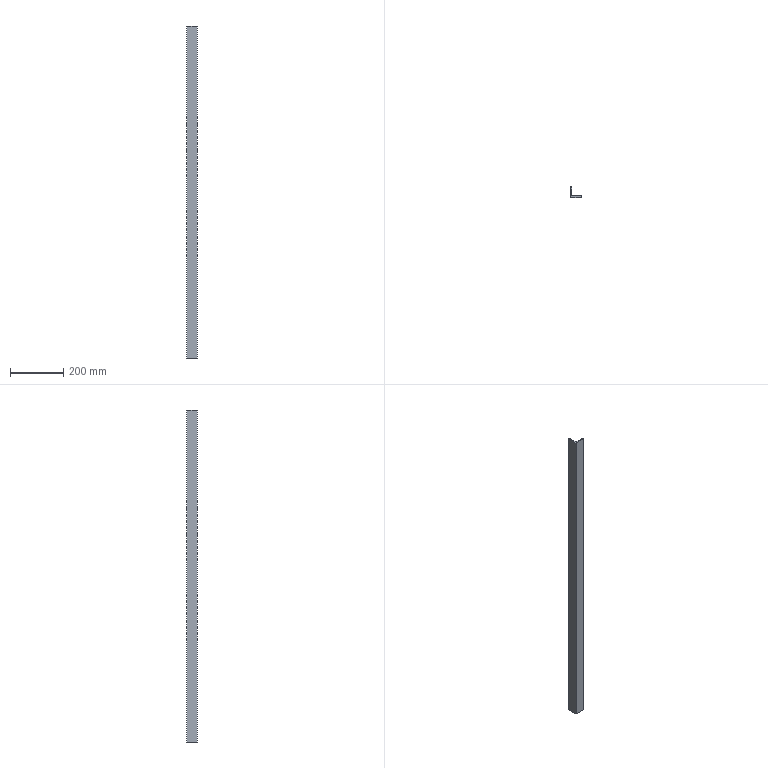Part | SolidWorks | features ICE 1, LibraryFeature 1 | 1 solid | 11 faces | box 40 x 40 x 1250 mm | volume 385753 mm3 | plane 8 | cylinder 3 | commonest cylinder face diameters 2.667 x2 10 x1
STEP:
#1=CARTESIAN_POINT('',(9.,4.,-625.));
#2=VERTEX_POINT('',#1);
#3=CARTESIAN_POINT('',(4.,9.,-625.));
#4=VERTEX_POINT('',#3);
#5=CARTESIAN_POINT('',(9.,9.,-625.));
#6=DIRECTION('',(0.,0.,-1.));
#7=DIRECTION('',(-1.,0.,0.));
#8=AXIS2_PLACEMENT_3D('',#5,#6,#7);
#9=CIRCLE('',#8,5.);
#10=EDGE_CURVE('',#2,#4,#9,.T.);
#11=ORIENTED_EDGE('',*,*,#10,.T.);
#12=CARTESIAN_POINT('',(4.,9.,625.));
#13=VERTEX_POINT('',#12);
#14=CARTESIAN_POINT('',(4.,9.,625.));
#15=DIRECTION('',(0.,0.,-1.));
#16=VECTOR('',#15,1000.);
#17=LINE('',#14,#16);
#18=EDGE_CURVE('',#13,#4,#17,.T.);
#19=ORIENTED_EDGE('',*,*,#18,.F.);
#20=CARTESIAN_POINT('',(9.,4.,625.));
#21=VERTEX_POINT('',#20);
#22=CARTESIAN_POINT('',(9.,9.,625.));
#23=DIRECTION('',(0.,0.,-1.));
#24=DIRECTION('',(-1.,0.,0.));
#25=AXIS2_PLACEMENT_3D('',#22,#23,#24);
#26=CIRCLE('',#25,5.);
#27=EDGE_CURVE('',#21,#13,#26,.T.);
#28=ORIENTED_EDGE('',*,*,#27,.F.);
#29=CARTESIAN_POINT('',(9.,4.,625.));
#30=DIRECTION('',(0.,0.,-1.));
#31=VECTOR('',#30,1000.);
#32=LINE('',#29,#31);
#33=EDGE_CURVE('',#21,#2,#32,.T.);
#34=ORIENTED_EDGE('',*,*,#33,.T.);
#35=EDGE_LOOP('',(#11,#19,#28,#34));
#36=FACE_OUTER_BOUND('',#35,.T.);
#37=CARTESIAN_POINT('',(9.,9.,625.));
#38=DIRECTION('',(0.,0.,-1.));
#39=DIRECTION('',(-1.,0.,0.));
#40=AXIS2_PLACEMENT_3D('',#37,#38,#39);
#41=CYLINDRICAL_SURFACE('',#40,5.);
#42=ADVANCED_FACE('',(#36),#41,.F.);
#43=CARTESIAN_POINT('',(4.,38.667,-625.));
#44=VERTEX_POINT('',#43);
#45=CARTESIAN_POINT('',(4.,38.667,-625.));
#46=DIRECTION('',(0.,-1.,0.));
#47=VECTOR('',#46,1000.);
#48=LINE('',#45,#47);
#49=EDGE_CURVE('',#44,#4,#48,.T.);
#50=ORIENTED_EDGE('',*,*,#49,.F.);
#51=CARTESIAN_POINT('',(4.,38.667,625.));
#52=VERTEX_POINT('',#51);
#53=CARTESIAN_POINT('',(4.,38.667,625.));
#54=DIRECTION('',(0.,0.,-1.));
#55=VECTOR('',#54,1000.);
#56=LINE('',#53,#55);
#57=EDGE_CURVE('',#52,#44,#56,.T.);
#58=ORIENTED_EDGE('',*,*,#57,.F.);
#59=CARTESIAN_POINT('',(4.,38.667,625.));
#60=DIRECTION('',(0.,-1.,0.));
#61=VECTOR('',#60,1000.);
#62=LINE('',#59,#61);
#63=EDGE_CURVE('',#52,#13,#62,.T.);
#64=ORIENTED_EDGE('',*,*,#63,.T.);
#65=ORIENTED_EDGE('',*,*,#18,.T.);
#66=EDGE_LOOP('',(#50,#58,#64,#65));
#67=FACE_OUTER_BOUND('',#66,.T.);
#68=CARTESIAN_POINT('',(4.,38.667,625.));
#69=DIRECTION('',(1.,0.,0.));
#70=DIRECTION('',(0.,1.,0.));
#71=AXIS2_PLACEMENT_3D('',#68,#69,#70);
#72=PLANE('',#71);
#73=ADVANCED_FACE('',(#67),#72,.T.);
#74=CARTESIAN_POINT('',(2.667,40.,-625.));
#75=VERTEX_POINT('',#74);
#76=CARTESIAN_POINT('',(2.667,38.667,-625.));
#77=DIRECTION('',(0.,0.,-1.));
#78=DIRECTION('',(-1.,0.,0.));
#79=AXIS2_PLACEMENT_3D('',#76,#77,#78);
#80=CIRCLE('',#79,1.333);
#81=EDGE_CURVE('',#75,#44,#80,.T.);
#82=ORIENTED_EDGE('',*,*,#81,.F.);
#83=CARTESIAN_POINT('',(2.667,40.,625.));
#84=VERTEX_POINT('',#83);
#85=CARTESIAN_POINT('',(2.667,40.,625.));
#86=DIRECTION('',(0.,0.,-1.));
#87=VECTOR('',#86,1000.);
#88=LINE('',#85,#87);
#89=EDGE_CURVE('',#84,#75,#88,.T.);
#90=ORIENTED_EDGE('',*,*,#89,.F.);
#91=CARTESIAN_POINT('',(2.667,38.667,625.));
#92=DIRECTION('',(0.,0.,-1.));
#93=DIRECTION('',(-1.,0.,0.));
#94=AXIS2_PLACEMENT_3D('',#91,#92,#93);
#95=CIRCLE('',#94,1.333);
#96=EDGE_CURVE('',#84,#52,#95,.T.);
#97=ORIENTED_EDGE('',*,*,#96,.T.);
#98=ORIENTED_EDGE('',*,*,#57,.T.);
#99=EDGE_LOOP('',(#82,#90,#97,#98));
#100=FACE_OUTER_BOUND('',#99,.T.);
#101=CARTESIAN_POINT('',(2.667,38.667,625.));
#102=DIRECTION('',(0.,0.,-1.));
#103=DIRECTION('',(-1.,0.,0.));
#104=AXIS2_PLACEMENT_3D('',#101,#102,#103);
#105=CYLINDRICAL_SURFACE('',#104,1.333);
#106=ADVANCED_FACE('',(#100),#105,.T.);
#107=CARTESIAN_POINT('',(0.,40.,-625.));
#108=VERTEX_POINT('',#107);
#109=CARTESIAN_POINT('',(0.,40.,-625.));
#110=DIRECTION('',(1.,0.,0.));
#111=VECTOR('',#110,1000.);
#112=LINE('',#109,#111);
#113=EDGE_CURVE('',#108,#75,#112,.T.);
#114=ORIENTED_EDGE('',*,*,#113,.F.);
#115=CARTESIAN_POINT('',(0.,40.,625.));
#116=VERTEX_POINT('',#115);
#117=CARTESIAN_POINT('',(0.,40.,625.));
#118=DIRECTION('',(0.,0.,-1.));
#119=VECTOR('',#118,1000.);
#120=LINE('',#117,#119);
#121=EDGE_CURVE('',#116,#108,#120,.T.);
#122=ORIENTED_EDGE('',*,*,#121,.F.);
#123=CARTESIAN_POINT('',(0.,40.,625.));
#124=DIRECTION('',(1.,0.,0.));
#125=VECTOR('',#124,1000.);
#126=LINE('',#123,#125);
#127=EDGE_CURVE('',#116,#84,#126,.T.);
#128=ORIENTED_EDGE('',*,*,#127,.T.);
#129=ORIENTED_EDGE('',*,*,#89,.T.);
#130=EDGE_LOOP('',(#114,#122,#128,#129));
#131=FACE_OUTER_BOUND('',#130,.T.);
#132=CARTESIAN_POINT('',(0.,40.,625.));
#133=DIRECTION('',(0.,1.,0.));
#134=DIRECTION('',(0.,0.,1.));
#135=AXIS2_PLACEMENT_3D('',#132,#133,#134);
#136=PLANE('',#135);
#137=ADVANCED_FACE('',(#131),#136,.T.);
#138=CARTESIAN_POINT('',(0.,0.,-625.));
#139=VERTEX_POINT('',#138);
#140=CARTESIAN_POINT('',(0.,0.,-625.));
#141=DIRECTION('',(0.,1.,0.));
#142=VECTOR('',#141,1000.);
#143=LINE('',#140,#142);
#144=EDGE_CURVE('',#139,#108,#143,.T.);
#145=ORIENTED_EDGE('',*,*,#144,.F.);
#146=CARTESIAN_POINT('',(0.,0.,625.));
#147=VERTEX_POINT('',#146);
#148=CARTESIAN_POINT('',(0.,0.,625.));
#149=DIRECTION('',(0.,0.,-1.));
#150=VECTOR('',#149,1000.);
#151=LINE('',#148,#150);
#152=EDGE_CURVE('',#147,#139,#151,.T.);
#153=ORIENTED_EDGE('',*,*,#152,.F.);
#154=CARTESIAN_POINT('',(0.,0.,625.));
#155=DIRECTION('',(0.,1.,0.));
#156=VECTOR('',#155,1000.);
#157=LINE('',#154,#156);
#158=EDGE_CURVE('',#147,#116,#157,.T.);
#159=ORIENTED_EDGE('',*,*,#158,.T.);
#160=ORIENTED_EDGE('',*,*,#121,.T.);
#161=EDGE_LOOP('',(#145,#153,#159,#160));
#162=FACE_OUTER_BOUND('',#161,.T.);
#163=CARTESIAN_POINT('',(0.,0.,625.));
#164=DIRECTION('',(-1.,0.,0.));
#165=DIRECTION('',(0.,0.,1.));
#166=AXIS2_PLACEMENT_3D('',#163,#164,#165);
#167=PLANE('',#166);
#168=ADVANCED_FACE('',(#162),#167,.T.);
#169=CARTESIAN_POINT('',(40.,0.,-625.));
#170=VERTEX_POINT('',#169);
#171=CARTESIAN_POINT('',(40.,0.,-625.));
#172=DIRECTION('',(-1.,0.,0.));
#173=VECTOR('',#172,1000.);
#174=LINE('',#171,#173);
#175=EDGE_CURVE('',#170,#139,#174,.T.);
#176=ORIENTED_EDGE('',*,*,#175,.F.);
#177=CARTESIAN_POINT('',(40.,0.,625.));
#178=VERTEX_POINT('',#177);
#179=CARTESIAN_POINT('',(40.,0.,625.));
#180=DIRECTION('',(0.,0.,-1.));
#181=VECTOR('',#180,1000.);
#182=LINE('',#179,#181);
#183=EDGE_CURVE('',#178,#170,#182,.T.);
#184=ORIENTED_EDGE('',*,*,#183,.F.);
#185=CARTESIAN_POINT('',(40.,0.,625.));
#186=DIRECTION('',(-1.,0.,0.));
#187=VECTOR('',#186,1000.);
#188=LINE('',#185,#187);
#189=EDGE_CURVE('',#178,#147,#188,.T.);
#190=ORIENTED_EDGE('',*,*,#189,.T.);
#191=ORIENTED_EDGE('',*,*,#152,.T.);
#192=EDGE_LOOP('',(#176,#184,#190,#191));
#193=FACE_OUTER_BOUND('',#192,.T.);
#194=CARTESIAN_POINT('',(40.,0.,625.));
#195=DIRECTION('',(0.,-1.,0.));
#196=DIRECTION('',(0.,0.,-1.));
#197=AXIS2_PLACEMENT_3D('',#194,#195,#196);
#198=PLANE('',#197);
#199=ADVANCED_FACE('',(#193),#198,.T.);
#200=CARTESIAN_POINT('',(40.,2.667,-625.));
#201=VERTEX_POINT('',#200);
#202=CARTESIAN_POINT('',(40.,0.,-625.));
#203=DIRECTION('',(0.,1.,0.));
#204=VECTOR('',#203,1000.);
#205=LINE('',#202,#204);
#206=EDGE_CURVE('',#170,#201,#205,.T.);
#207=ORIENTED_EDGE('',*,*,#206,.T.);
#208=CARTESIAN_POINT('',(40.,2.667,625.));
#209=VERTEX_POINT('',#208);
#210=CARTESIAN_POINT('',(40.,2.667,625.));
#211=DIRECTION('',(0.,0.,-1.));
#212=VECTOR('',#211,1000.);
#213=LINE('',#210,#212);
#214=EDGE_CURVE('',#209,#201,#213,.T.);
#215=ORIENTED_EDGE('',*,*,#214,.F.);
#216=CARTESIAN_POINT('',(40.,0.,625.));
#217=DIRECTION('',(0.,1.,0.));
#218=VECTOR('',#217,1000.);
#219=LINE('',#216,#218);
#220=EDGE_CURVE('',#178,#209,#219,.T.);
#221=ORIENTED_EDGE('',*,*,#220,.F.);
#222=ORIENTED_EDGE('',*,*,#183,.T.);
#223=EDGE_LOOP('',(#207,#215,#221,#222));
#224=FACE_OUTER_BOUND('',#223,.T.);
#225=CARTESIAN_POINT('',(40.,0.,625.));
#226=DIRECTION('',(-1.,0.,0.));
#227=DIRECTION('',(0.,0.,1.));
#228=AXIS2_PLACEMENT_3D('',#225,#226,#227);
#229=PLANE('',#228);
#230=ADVANCED_FACE('',(#224),#229,.F.);
#231=CARTESIAN_POINT('',(38.667,4.,-625.));
#232=VERTEX_POINT('',#231);
#233=CARTESIAN_POINT('',(38.667,2.667,-625.));
#234=DIRECTION('',(0.,0.,1.));
#235=DIRECTION('',(1.,0.,0.));
#236=AXIS2_PLACEMENT_3D('',#233,#234,#235);
#237=CIRCLE('',#236,1.333);
#238=EDGE_CURVE('',#201,#232,#237,.T.);
#239=ORIENTED_EDGE('',*,*,#238,.T.);
#240=CARTESIAN_POINT('',(38.667,4.,625.));
#241=VERTEX_POINT('',#240);
#242=CARTESIAN_POINT('',(38.667,4.,625.));
#243=DIRECTION('',(0.,0.,-1.));
#244=VECTOR('',#243,1000.);
#245=LINE('',#242,#244);
#246=EDGE_CURVE('',#241,#232,#245,.T.);
#247=ORIENTED_EDGE('',*,*,#246,.F.);
#248=CARTESIAN_POINT('',(38.667,2.667,625.));
#249=DIRECTION('',(0.,0.,1.));
#250=DIRECTION('',(1.,0.,0.));
#251=AXIS2_PLACEMENT_3D('',#248,#249,#250);
#252=CIRCLE('',#251,1.333);
#253=EDGE_CURVE('',#209,#241,#252,.T.);
#254=ORIENTED_EDGE('',*,*,#253,.F.);
#255=ORIENTED_EDGE('',*,*,#214,.T.);
#256=EDGE_LOOP('',(#239,#247,#254,#255));
#257=FACE_OUTER_BOUND('',#256,.T.);
#258=CARTESIAN_POINT('',(38.667,2.667,625.));
#259=DIRECTION('',(0.,0.,-1.));
#260=DIRECTION('',(-1.,0.,0.));
#261=AXIS2_PLACEMENT_3D('',#258,#259,#260);
#262=CYLINDRICAL_SURFACE('',#261,1.333);
#263=ADVANCED_FACE('',(#257),#262,.T.);
#264=CARTESIAN_POINT('',(9.,4.,-625.));
#265=DIRECTION('',(1.,0.,0.));
#266=VECTOR('',#265,1000.);
#267=LINE('',#264,#266);
#268=EDGE_CURVE('',#2,#232,#267,.T.);
#269=ORIENTED_EDGE('',*,*,#268,.F.);
#270=ORIENTED_EDGE('',*,*,#33,.F.);
#271=CARTESIAN_POINT('',(9.,4.,625.));
#272=DIRECTION('',(1.,0.,0.));
#273=VECTOR('',#272,1000.);
#274=LINE('',#271,#273);
#275=EDGE_CURVE('',#21,#241,#274,.T.);
#276=ORIENTED_EDGE('',*,*,#275,.T.);
#277=ORIENTED_EDGE('',*,*,#246,.T.);
#278=EDGE_LOOP('',(#269,#270,#276,#277));
#279=FACE_OUTER_BOUND('',#278,.T.);
#280=CARTESIAN_POINT('',(9.,4.,625.));
#281=DIRECTION('',(0.,1.,0.));
#282=DIRECTION('',(0.,0.,1.));
#283=AXIS2_PLACEMENT_3D('',#280,#281,#282);
#284=PLANE('',#283);
#285=ADVANCED_FACE('',(#279),#284,.T.);
#286=ORIENTED_EDGE('',*,*,#27,.T.);
#287=ORIENTED_EDGE('',*,*,#63,.F.);
#288=ORIENTED_EDGE('',*,*,#96,.F.);
#289=ORIENTED_EDGE('',*,*,#127,.F.);
#290=ORIENTED_EDGE('',*,*,#158,.F.);
#291=ORIENTED_EDGE('',*,*,#189,.F.);
#292=ORIENTED_EDGE('',*,*,#220,.T.);
#293=ORIENTED_EDGE('',*,*,#253,.T.);
#294=ORIENTED_EDGE('',*,*,#275,.F.);
#295=EDGE_LOOP('',(#286,#287,#288,#289,#290,#291,#292,#293,#294));
#296=FACE_OUTER_BOUND('',#295,.T.);
#297=CARTESIAN_POINT('',(9.,9.,625.));
#298=DIRECTION('',(0.,0.,-1.));
#299=DIRECTION('',(-1.,0.,0.));
#300=AXIS2_PLACEMENT_3D('',#297,#298,#299);
#301=PLANE('',#300);
#302=ADVANCED_FACE('',(#296),#301,.F.);
#303=ORIENTED_EDGE('',*,*,#10,.F.);
#304=ORIENTED_EDGE('',*,*,#268,.T.);
#305=ORIENTED_EDGE('',*,*,#238,.F.);
#306=ORIENTED_EDGE('',*,*,#206,.F.);
#307=ORIENTED_EDGE('',*,*,#175,.T.);
#308=ORIENTED_EDGE('',*,*,#144,.T.);
#309=ORIENTED_EDGE('',*,*,#113,.T.);
#310=ORIENTED_EDGE('',*,*,#81,.T.);
#311=ORIENTED_EDGE('',*,*,#49,.T.);
#312=EDGE_LOOP('',(#303,#304,#305,#306,#307,#308,#309,#310,#311));
#313=FACE_OUTER_BOUND('',#312,.T.);
#314=CARTESIAN_POINT('',(9.,9.,-625.));
#315=DIRECTION('',(0.,0.,-1.));
#316=DIRECTION('',(-1.,0.,0.));
#317=AXIS2_PLACEMENT_3D('',#314,#315,#316);
#318=PLANE('',#317);
#319=ADVANCED_FACE('',(#313),#318,.T.);
#320=CLOSED_SHELL('',(#42,#73,#106,#137,#168,#199,#230,#263,#285,#302,#319));
#321=MANIFOLD_SOLID_BREP('',#320);
#322=CARTESIAN_POINT('',(0.,0.,0.));
#323=DIRECTION('',(0.,0.,1.));
#324=DIRECTION('',(1.,0.,0.));
#325=AXIS2_PLACEMENT_3D('',#322,#323,#324);
#326=(LENGTH_UNIT()NAMED_UNIT(*)SI_UNIT(.MILLI.,.METRE.));
#327=UNCERTAINTY_MEASURE_WITH_UNIT(LENGTH_MEASURE(0.00001),#326,'','');
#328=(NAMED_UNIT(*)PLANE_ANGLE_UNIT()SI_UNIT($,.RADIAN.));
#329=(NAMED_UNIT(*)SI_UNIT($,.STERADIAN.)SOLID_ANGLE_UNIT());
#330=(GEOMETRIC_REPRESENTATION_CONTEXT(3)GLOBAL_UNCERTAINTY_ASSIGNED_CONTEXT((#327))GLOBAL_UNIT_ASSIGNED_CONTEXT((#326,#328,#329))REPRESENTATION_CONTEXT('',''));
#331=ADVANCED_BREP_SHAPE_REPRESENTATION('',(#321,#325),#330);